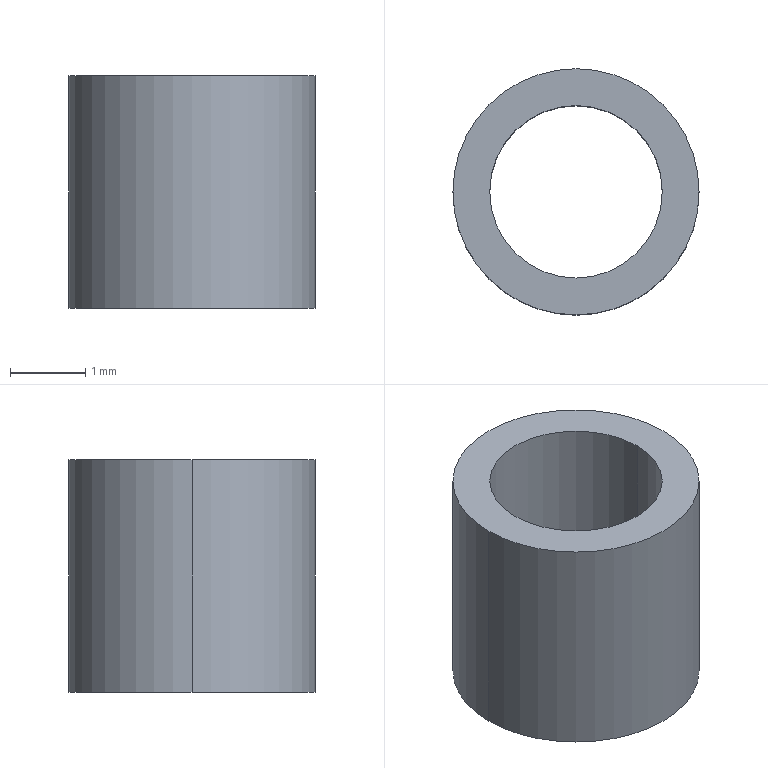Part | SolidWorks | features Extrusion 1 | 1 solid | 6 faces | box 3.28 x 3.28 x 3.1 mm | volume 13.314 mm3 | cylinder 4 | plane 2 | commonest cylinder face diameters 2.3 x2 3.28 x2
STEP:
#1=CARTESIAN_POINT('',(-1.15,0.,3.1));
#2=VERTEX_POINT('',#1);
#3=CARTESIAN_POINT('',(1.15,0.,3.1));
#4=VERTEX_POINT('',#3);
#5=CARTESIAN_POINT('',(0.,0.,3.1));
#6=DIRECTION('',(0.,0.,1.));
#7=DIRECTION('',(1.,0.,0.));
#8=AXIS2_PLACEMENT_3D('',#5,#6,#7);
#9=CIRCLE('',#8,1.15);
#10=EDGE_CURVE('',#2,#4,#9,.T.);
#11=ORIENTED_EDGE('',*,*,#10,.T.);
#12=CARTESIAN_POINT('',(1.15,0.,0.));
#13=VERTEX_POINT('',#12);
#14=CARTESIAN_POINT('',(1.15,0.,3.1));
#15=DIRECTION('',(0.,0.,-1.));
#16=VECTOR('',#15,1000.);
#17=LINE('',#14,#16);
#18=EDGE_CURVE('',#4,#13,#17,.T.);
#19=ORIENTED_EDGE('',*,*,#18,.T.);
#20=CARTESIAN_POINT('',(-1.15,0.,0.));
#21=VERTEX_POINT('',#20);
#22=CARTESIAN_POINT('',(0.,0.,0.));
#23=DIRECTION('',(0.,0.,1.));
#24=DIRECTION('',(1.,0.,0.));
#25=AXIS2_PLACEMENT_3D('',#22,#23,#24);
#26=CIRCLE('',#25,1.15);
#27=EDGE_CURVE('',#21,#13,#26,.T.);
#28=ORIENTED_EDGE('',*,*,#27,.F.);
#29=CARTESIAN_POINT('',(-1.15,0.,3.1));
#30=DIRECTION('',(0.,0.,-1.));
#31=VECTOR('',#30,1000.);
#32=LINE('',#29,#31);
#33=EDGE_CURVE('',#2,#21,#32,.T.);
#34=ORIENTED_EDGE('',*,*,#33,.F.);
#35=EDGE_LOOP('',(#11,#19,#28,#34));
#36=FACE_OUTER_BOUND('',#35,.T.);
#37=CARTESIAN_POINT('',(0.,0.,3.1));
#38=DIRECTION('',(0.,0.,-1.));
#39=DIRECTION('',(-1.,0.,0.));
#40=AXIS2_PLACEMENT_3D('',#37,#38,#39);
#41=CYLINDRICAL_SURFACE('',#40,1.15);
#42=ADVANCED_FACE('',(#36),#41,.F.);
#43=CARTESIAN_POINT('',(1.64,0.,3.1));
#44=VERTEX_POINT('',#43);
#45=CARTESIAN_POINT('',(-1.64,0.,3.1));
#46=VERTEX_POINT('',#45);
#47=CARTESIAN_POINT('',(0.,0.,3.1));
#48=DIRECTION('',(0.,0.,1.));
#49=DIRECTION('',(1.,0.,0.));
#50=AXIS2_PLACEMENT_3D('',#47,#48,#49);
#51=CIRCLE('',#50,1.64);
#52=EDGE_CURVE('',#44,#46,#51,.T.);
#53=ORIENTED_EDGE('',*,*,#52,.F.);
#54=CARTESIAN_POINT('',(1.64,0.,0.));
#55=VERTEX_POINT('',#54);
#56=CARTESIAN_POINT('',(1.64,0.,3.1));
#57=DIRECTION('',(0.,0.,-1.));
#58=VECTOR('',#57,1000.);
#59=LINE('',#56,#58);
#60=EDGE_CURVE('',#44,#55,#59,.T.);
#61=ORIENTED_EDGE('',*,*,#60,.T.);
#62=CARTESIAN_POINT('',(-1.64,0.,0.));
#63=VERTEX_POINT('',#62);
#64=CARTESIAN_POINT('',(0.,0.,0.));
#65=DIRECTION('',(0.,0.,1.));
#66=DIRECTION('',(1.,0.,0.));
#67=AXIS2_PLACEMENT_3D('',#64,#65,#66);
#68=CIRCLE('',#67,1.64);
#69=EDGE_CURVE('',#55,#63,#68,.T.);
#70=ORIENTED_EDGE('',*,*,#69,.T.);
#71=CARTESIAN_POINT('',(-1.64,0.,3.1));
#72=DIRECTION('',(0.,0.,-1.));
#73=VECTOR('',#72,1000.);
#74=LINE('',#71,#73);
#75=EDGE_CURVE('',#46,#63,#74,.T.);
#76=ORIENTED_EDGE('',*,*,#75,.F.);
#77=EDGE_LOOP('',(#53,#61,#70,#76));
#78=FACE_OUTER_BOUND('',#77,.T.);
#79=CARTESIAN_POINT('',(0.,0.,3.1));
#80=DIRECTION('',(0.,0.,-1.));
#81=DIRECTION('',(-1.,0.,0.));
#82=AXIS2_PLACEMENT_3D('',#79,#80,#81);
#83=CYLINDRICAL_SURFACE('',#82,1.64);
#84=ADVANCED_FACE('',(#78),#83,.T.);
#85=CARTESIAN_POINT('',(0.,0.,3.1));
#86=DIRECTION('',(0.,0.,1.));
#87=DIRECTION('',(1.,0.,0.));
#88=AXIS2_PLACEMENT_3D('',#85,#86,#87);
#89=CIRCLE('',#88,1.64);
#90=EDGE_CURVE('',#46,#44,#89,.T.);
#91=ORIENTED_EDGE('',*,*,#90,.T.);
#92=ORIENTED_EDGE('',*,*,#52,.T.);
#93=EDGE_LOOP('',(#91,#92));
#94=FACE_OUTER_BOUND('',#93,.T.);
#95=ORIENTED_EDGE('',*,*,#10,.F.);
#96=CARTESIAN_POINT('',(0.,0.,3.1));
#97=DIRECTION('',(0.,0.,1.));
#98=DIRECTION('',(1.,0.,0.));
#99=AXIS2_PLACEMENT_3D('',#96,#97,#98);
#100=CIRCLE('',#99,1.15);
#101=EDGE_CURVE('',#4,#2,#100,.T.);
#102=ORIENTED_EDGE('',*,*,#101,.F.);
#103=EDGE_LOOP('',(#95,#102));
#104=FACE_BOUND('',#103,.T.);
#105=CARTESIAN_POINT('',(0.,0.,3.1));
#106=DIRECTION('',(0.,0.,1.));
#107=DIRECTION('',(1.,0.,0.));
#108=AXIS2_PLACEMENT_3D('',#105,#106,#107);
#109=PLANE('',#108);
#110=ADVANCED_FACE('',(#94,#104),#109,.T.);
#111=CARTESIAN_POINT('',(0.,0.,0.));
#112=DIRECTION('',(0.,0.,1.));
#113=DIRECTION('',(1.,0.,0.));
#114=AXIS2_PLACEMENT_3D('',#111,#112,#113);
#115=CIRCLE('',#114,1.64);
#116=EDGE_CURVE('',#63,#55,#115,.T.);
#117=ORIENTED_EDGE('',*,*,#116,.F.);
#118=ORIENTED_EDGE('',*,*,#69,.F.);
#119=EDGE_LOOP('',(#117,#118));
#120=FACE_OUTER_BOUND('',#119,.T.);
#121=ORIENTED_EDGE('',*,*,#27,.T.);
#122=CARTESIAN_POINT('',(0.,0.,0.));
#123=DIRECTION('',(0.,0.,1.));
#124=DIRECTION('',(1.,0.,0.));
#125=AXIS2_PLACEMENT_3D('',#122,#123,#124);
#126=CIRCLE('',#125,1.15);
#127=EDGE_CURVE('',#13,#21,#126,.T.);
#128=ORIENTED_EDGE('',*,*,#127,.T.);
#129=EDGE_LOOP('',(#121,#128));
#130=FACE_BOUND('',#129,.T.);
#131=CARTESIAN_POINT('',(0.,0.,0.));
#132=DIRECTION('',(0.,0.,1.));
#133=DIRECTION('',(1.,0.,0.));
#134=AXIS2_PLACEMENT_3D('',#131,#132,#133);
#135=PLANE('',#134);
#136=ADVANCED_FACE('',(#120,#130),#135,.F.);
#137=ORIENTED_EDGE('',*,*,#60,.F.);
#138=ORIENTED_EDGE('',*,*,#90,.F.);
#139=ORIENTED_EDGE('',*,*,#75,.T.);
#140=ORIENTED_EDGE('',*,*,#116,.T.);
#141=EDGE_LOOP('',(#137,#138,#139,#140));
#142=FACE_OUTER_BOUND('',#141,.T.);
#143=CARTESIAN_POINT('',(0.,0.,3.1));
#144=DIRECTION('',(0.,0.,-1.));
#145=DIRECTION('',(-1.,0.,0.));
#146=AXIS2_PLACEMENT_3D('',#143,#144,#145);
#147=CYLINDRICAL_SURFACE('',#146,1.64);
#148=ADVANCED_FACE('',(#142),#147,.T.);
#149=ORIENTED_EDGE('',*,*,#18,.F.);
#150=ORIENTED_EDGE('',*,*,#101,.T.);
#151=ORIENTED_EDGE('',*,*,#33,.T.);
#152=ORIENTED_EDGE('',*,*,#127,.F.);
#153=EDGE_LOOP('',(#149,#150,#151,#152));
#154=FACE_OUTER_BOUND('',#153,.T.);
#155=CARTESIAN_POINT('',(0.,0.,3.1));
#156=DIRECTION('',(0.,0.,-1.));
#157=DIRECTION('',(-1.,0.,0.));
#158=AXIS2_PLACEMENT_3D('',#155,#156,#157);
#159=CYLINDRICAL_SURFACE('',#158,1.15);
#160=ADVANCED_FACE('',(#154),#159,.F.);
#161=CLOSED_SHELL('',(#42,#84,#110,#136,#148,#160));
#162=MANIFOLD_SOLID_BREP('',#161);
#163=CARTESIAN_POINT('',(0.,0.,0.));
#164=DIRECTION('',(0.,0.,1.));
#165=DIRECTION('',(1.,0.,0.));
#166=AXIS2_PLACEMENT_3D('',#163,#164,#165);
#167=(LENGTH_UNIT()NAMED_UNIT(*)SI_UNIT(.MILLI.,.METRE.));
#168=UNCERTAINTY_MEASURE_WITH_UNIT(LENGTH_MEASURE(0.00001),#167,'','');
#169=(NAMED_UNIT(*)PLANE_ANGLE_UNIT()SI_UNIT($,.RADIAN.));
#170=(NAMED_UNIT(*)SI_UNIT($,.STERADIAN.)SOLID_ANGLE_UNIT());
#171=(GEOMETRIC_REPRESENTATION_CONTEXT(3)GLOBAL_UNCERTAINTY_ASSIGNED_CONTEXT((#168))GLOBAL_UNIT_ASSIGNED_CONTEXT((#167,#169,#170))REPRESENTATION_CONTEXT('',''));
#172=ADVANCED_BREP_SHAPE_REPRESENTATION('',(#162,#166),#171);